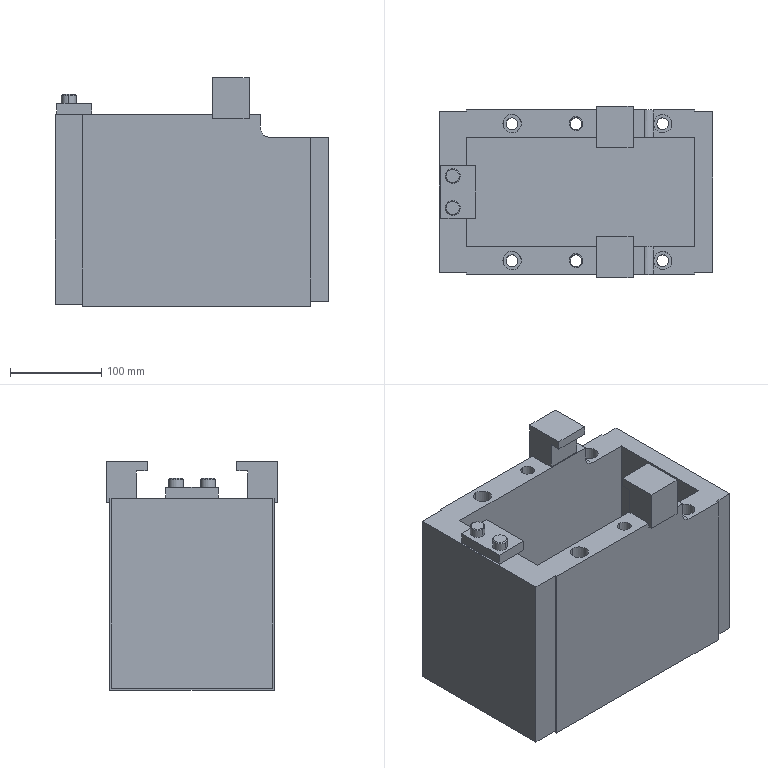Part | NX | features solid 2 | 1 solid | 88 faces | box 300 x 188 x 250 mm | volume 5968535 mm3 | plane 53 | cylinder 30 | cone 4 | spline 1 | commonest cylinder face diameters 13 x12 20 x10 15 x4 16.25 x4